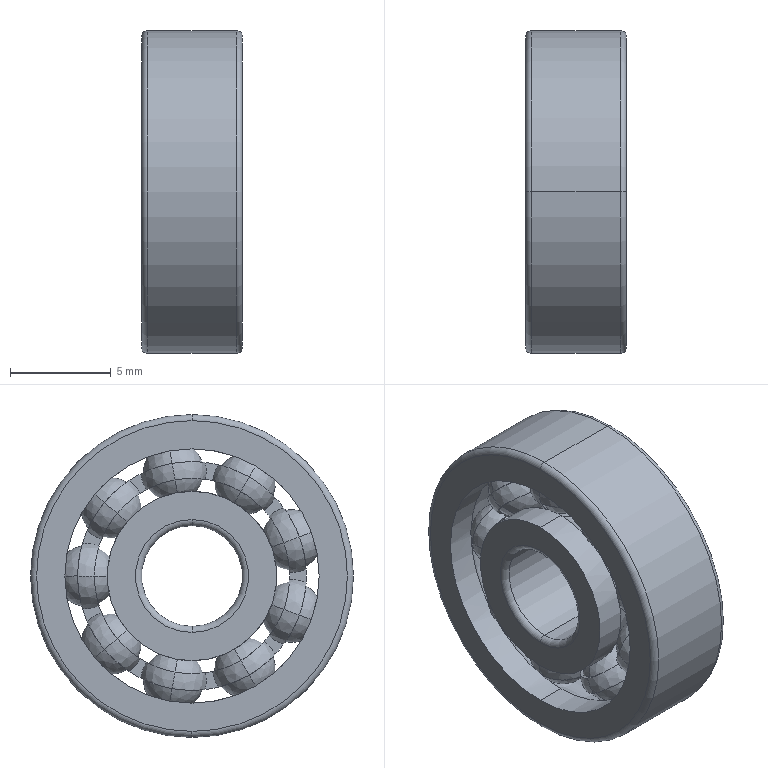Part | NX | features BREP 1 | 1 solid | 148 faces | box 5 x 16 x 16 mm | volume 656.874 mm3 | sphere 72 | torus 38 | plane 22 | cylinder 16 | commonest cylinder face diameters 8.4 x4 12.6 x4 5 x2 9.675 x2 11.325 x2 16 x2